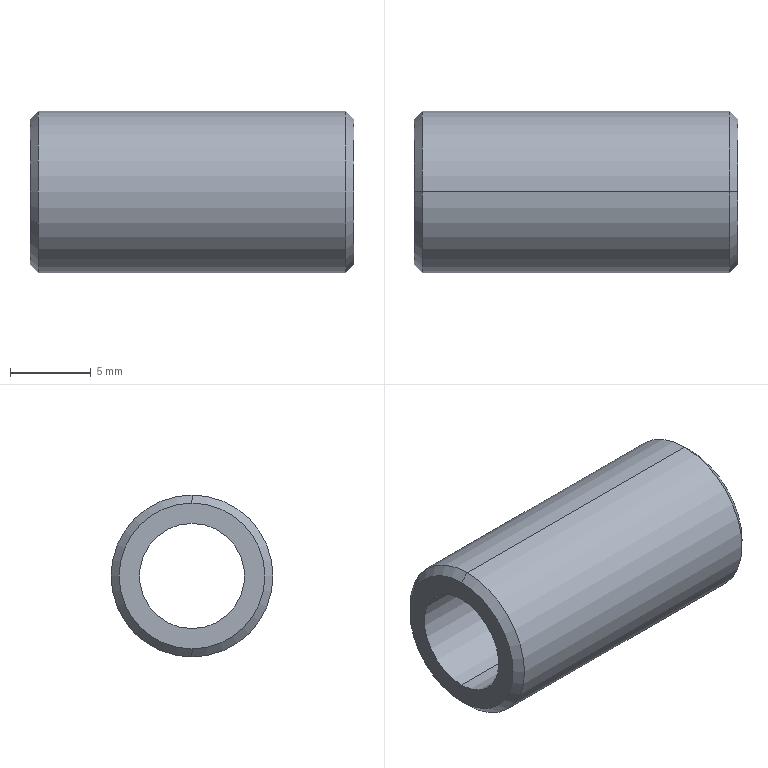Part | SolidWorks | features Chamfer 1, Extrusion 1, ICE 1 | 1 solid | 10 faces | box 20 x 10 x 10 mm | volume 899.543 mm3 | cylinder 4 | cone 4 | plane 2 | commonest cylinder face diameters 6.5 x2 10 x2
STEP:
#1=CARTESIAN_POINT('',(20.,0.,-3.25));
#2=VERTEX_POINT('',#1);
#3=CARTESIAN_POINT('',(20.,0.,3.25));
#4=VERTEX_POINT('',#3);
#5=CARTESIAN_POINT('',(20.,0.,0.));
#6=DIRECTION('',(-1.,0.,0.));
#7=DIRECTION('',(0.,0.,1.));
#8=AXIS2_PLACEMENT_3D('',#5,#6,#7);
#9=CIRCLE('',#8,3.25);
#10=EDGE_CURVE('',#2,#4,#9,.T.);
#11=ORIENTED_EDGE('',*,*,#10,.F.);
#12=CARTESIAN_POINT('',(0.,0.,-3.25));
#13=VERTEX_POINT('',#12);
#14=CARTESIAN_POINT('',(20.,0.,-3.25));
#15=DIRECTION('',(-1.,0.,0.));
#16=VECTOR('',#15,1000.);
#17=LINE('',#14,#16);
#18=EDGE_CURVE('',#2,#13,#17,.T.);
#19=ORIENTED_EDGE('',*,*,#18,.T.);
#20=CARTESIAN_POINT('',(0.,0.,3.25));
#21=VERTEX_POINT('',#20);
#22=CARTESIAN_POINT('',(0.,0.,0.));
#23=DIRECTION('',(-1.,0.,0.));
#24=DIRECTION('',(0.,0.,1.));
#25=AXIS2_PLACEMENT_3D('',#22,#23,#24);
#26=CIRCLE('',#25,3.25);
#27=EDGE_CURVE('',#13,#21,#26,.T.);
#28=ORIENTED_EDGE('',*,*,#27,.T.);
#29=CARTESIAN_POINT('',(20.,0.,3.25));
#30=DIRECTION('',(-1.,0.,0.));
#31=VECTOR('',#30,1000.);
#32=LINE('',#29,#31);
#33=EDGE_CURVE('',#4,#21,#32,.T.);
#34=ORIENTED_EDGE('',*,*,#33,.F.);
#35=EDGE_LOOP('',(#11,#19,#28,#34));
#36=FACE_OUTER_BOUND('',#35,.T.);
#37=CARTESIAN_POINT('',(20.,0.,0.));
#38=DIRECTION('',(-1.,0.,0.));
#39=DIRECTION('',(0.,0.,1.));
#40=AXIS2_PLACEMENT_3D('',#37,#38,#39);
#41=CYLINDRICAL_SURFACE('',#40,3.25);
#42=ADVANCED_FACE('',(#36),#41,.F.);
#43=CARTESIAN_POINT('',(20.,0.,-4.5));
#44=VERTEX_POINT('',#43);
#45=CARTESIAN_POINT('',(20.,0.,4.5));
#46=VERTEX_POINT('',#45);
#47=CARTESIAN_POINT('',(20.,0.,0.));
#48=DIRECTION('',(1.,0.,0.));
#49=DIRECTION('',(0.,0.,-1.));
#50=AXIS2_PLACEMENT_3D('',#47,#48,#49);
#51=CIRCLE('',#50,4.5);
#52=EDGE_CURVE('',#44,#46,#51,.T.);
#53=ORIENTED_EDGE('',*,*,#52,.F.);
#54=CARTESIAN_POINT('',(19.5,0.,-5.));
#55=VERTEX_POINT('',#54);
#56=CARTESIAN_POINT('',(20.,0.,-4.5));
#57=DIRECTION('',(-0.7071,0.,-0.7071));
#58=VECTOR('',#57,1000.);
#59=LINE('',#56,#58);
#60=EDGE_CURVE('',#44,#55,#59,.T.);
#61=ORIENTED_EDGE('',*,*,#60,.T.);
#62=CARTESIAN_POINT('',(19.5,0.,5.));
#63=VERTEX_POINT('',#62);
#64=CARTESIAN_POINT('',(19.5,0.,0.));
#65=DIRECTION('',(-1.,0.,0.));
#66=DIRECTION('',(0.,0.,-1.));
#67=AXIS2_PLACEMENT_3D('',#64,#65,#66);
#68=CIRCLE('',#67,5.);
#69=EDGE_CURVE('',#63,#55,#68,.T.);
#70=ORIENTED_EDGE('',*,*,#69,.F.);
#71=CARTESIAN_POINT('',(20.,0.,4.5));
#72=DIRECTION('',(-0.7071,0.,0.7071));
#73=VECTOR('',#72,1000.);
#74=LINE('',#71,#73);
#75=EDGE_CURVE('',#46,#63,#74,.T.);
#76=ORIENTED_EDGE('',*,*,#75,.F.);
#77=EDGE_LOOP('',(#53,#61,#70,#76));
#78=FACE_OUTER_BOUND('',#77,.T.);
#79=CARTESIAN_POINT('',(20.,0.,0.));
#80=DIRECTION('',(-1.,0.,0.));
#81=DIRECTION('',(0.,0.,1.));
#82=AXIS2_PLACEMENT_3D('',#79,#80,#81);
#83=CONICAL_SURFACE('',#82,4.5,0.7854);
#84=ADVANCED_FACE('',(#78),#83,.T.);
#85=CARTESIAN_POINT('',(0.,0.,4.5));
#86=VERTEX_POINT('',#85);
#87=CARTESIAN_POINT('',(0.,0.,-4.5));
#88=VERTEX_POINT('',#87);
#89=CARTESIAN_POINT('',(0.,0.,0.));
#90=DIRECTION('',(-1.,0.,0.));
#91=DIRECTION('',(0.,0.,-1.));
#92=AXIS2_PLACEMENT_3D('',#89,#90,#91);
#93=CIRCLE('',#92,4.5);
#94=EDGE_CURVE('',#86,#88,#93,.T.);
#95=ORIENTED_EDGE('',*,*,#94,.F.);
#96=CARTESIAN_POINT('',(0.5,0.,5.));
#97=VERTEX_POINT('',#96);
#98=CARTESIAN_POINT('',(0.5,0.,5.));
#99=DIRECTION('',(0.7071,0.,0.7071));
#100=VECTOR('',#99,1000.);
#101=LINE('',#98,#100);
#102=EDGE_CURVE('',#86,#97,#101,.T.);
#103=ORIENTED_EDGE('',*,*,#102,.T.);
#104=CARTESIAN_POINT('',(0.5,0.,-5.));
#105=VERTEX_POINT('',#104);
#106=CARTESIAN_POINT('',(0.5,0.,0.));
#107=DIRECTION('',(1.,0.,0.));
#108=DIRECTION('',(0.,0.,-1.));
#109=AXIS2_PLACEMENT_3D('',#106,#107,#108);
#110=CIRCLE('',#109,5.);
#111=EDGE_CURVE('',#105,#97,#110,.T.);
#112=ORIENTED_EDGE('',*,*,#111,.F.);
#113=CARTESIAN_POINT('',(0.5,0.,-5.));
#114=DIRECTION('',(0.7071,0.,-0.7071));
#115=VECTOR('',#114,1000.);
#116=LINE('',#113,#115);
#117=EDGE_CURVE('',#88,#105,#116,.T.);
#118=ORIENTED_EDGE('',*,*,#117,.F.);
#119=EDGE_LOOP('',(#95,#103,#112,#118));
#120=FACE_OUTER_BOUND('',#119,.T.);
#121=CARTESIAN_POINT('',(0.5,0.,0.));
#122=DIRECTION('',(1.,0.,0.));
#123=DIRECTION('',(0.,0.,-1.));
#124=AXIS2_PLACEMENT_3D('',#121,#122,#123);
#125=CONICAL_SURFACE('',#124,5.,0.7854);
#126=ADVANCED_FACE('',(#120),#125,.T.);
#127=ORIENTED_EDGE('',*,*,#69,.T.);
#128=CARTESIAN_POINT('',(20.,0.,-5.));
#129=DIRECTION('',(-1.,0.,0.));
#130=VECTOR('',#129,1000.);
#131=LINE('',#128,#130);
#132=EDGE_CURVE('',#55,#105,#131,.T.);
#133=ORIENTED_EDGE('',*,*,#132,.T.);
#134=ORIENTED_EDGE('',*,*,#111,.T.);
#135=CARTESIAN_POINT('',(20.,0.,5.));
#136=DIRECTION('',(-1.,0.,0.));
#137=VECTOR('',#136,1000.);
#138=LINE('',#135,#137);
#139=EDGE_CURVE('',#63,#97,#138,.T.);
#140=ORIENTED_EDGE('',*,*,#139,.F.);
#141=EDGE_LOOP('',(#127,#133,#134,#140));
#142=FACE_OUTER_BOUND('',#141,.T.);
#143=CARTESIAN_POINT('',(20.,0.,0.));
#144=DIRECTION('',(-1.,0.,0.));
#145=DIRECTION('',(0.,0.,1.));
#146=AXIS2_PLACEMENT_3D('',#143,#144,#145);
#147=CYLINDRICAL_SURFACE('',#146,5.);
#148=ADVANCED_FACE('',(#142),#147,.T.);
#149=ORIENTED_EDGE('',*,*,#132,.F.);
#150=CARTESIAN_POINT('',(19.5,0.,0.));
#151=DIRECTION('',(-1.,0.,0.));
#152=DIRECTION('',(0.,0.,-1.));
#153=AXIS2_PLACEMENT_3D('',#150,#151,#152);
#154=CIRCLE('',#153,5.);
#155=EDGE_CURVE('',#55,#63,#154,.T.);
#156=ORIENTED_EDGE('',*,*,#155,.T.);
#157=ORIENTED_EDGE('',*,*,#139,.T.);
#158=CARTESIAN_POINT('',(0.5,0.,0.));
#159=DIRECTION('',(1.,0.,0.));
#160=DIRECTION('',(0.,0.,-1.));
#161=AXIS2_PLACEMENT_3D('',#158,#159,#160);
#162=CIRCLE('',#161,5.);
#163=EDGE_CURVE('',#97,#105,#162,.T.);
#164=ORIENTED_EDGE('',*,*,#163,.T.);
#165=EDGE_LOOP('',(#149,#156,#157,#164));
#166=FACE_OUTER_BOUND('',#165,.T.);
#167=CARTESIAN_POINT('',(20.,0.,0.));
#168=DIRECTION('',(-1.,0.,0.));
#169=DIRECTION('',(0.,0.,1.));
#170=AXIS2_PLACEMENT_3D('',#167,#168,#169);
#171=CYLINDRICAL_SURFACE('',#170,5.);
#172=ADVANCED_FACE('',(#166),#171,.T.);
#173=CARTESIAN_POINT('',(20.,0.,0.));
#174=DIRECTION('',(-1.,0.,0.));
#175=DIRECTION('',(0.,0.,1.));
#176=AXIS2_PLACEMENT_3D('',#173,#174,#175);
#177=CIRCLE('',#176,3.25);
#178=EDGE_CURVE('',#4,#2,#177,.T.);
#179=ORIENTED_EDGE('',*,*,#178,.T.);
#180=ORIENTED_EDGE('',*,*,#10,.T.);
#181=EDGE_LOOP('',(#179,#180));
#182=FACE_BOUND('',#181,.T.);
#183=CARTESIAN_POINT('',(20.,0.,0.));
#184=DIRECTION('',(1.,0.,0.));
#185=DIRECTION('',(0.,0.,-1.));
#186=AXIS2_PLACEMENT_3D('',#183,#184,#185);
#187=CIRCLE('',#186,4.5);
#188=EDGE_CURVE('',#46,#44,#187,.T.);
#189=ORIENTED_EDGE('',*,*,#188,.T.);
#190=ORIENTED_EDGE('',*,*,#52,.T.);
#191=EDGE_LOOP('',(#189,#190));
#192=FACE_OUTER_BOUND('',#191,.T.);
#193=CARTESIAN_POINT('',(20.,0.,0.));
#194=DIRECTION('',(1.,0.,0.));
#195=DIRECTION('',(0.,0.,-1.));
#196=AXIS2_PLACEMENT_3D('',#193,#194,#195);
#197=PLANE('',#196);
#198=ADVANCED_FACE('',(#182,#192),#197,.T.);
#199=CARTESIAN_POINT('',(0.,0.,0.));
#200=DIRECTION('',(-1.,0.,0.));
#201=DIRECTION('',(0.,0.,1.));
#202=AXIS2_PLACEMENT_3D('',#199,#200,#201);
#203=CIRCLE('',#202,3.25);
#204=EDGE_CURVE('',#21,#13,#203,.T.);
#205=ORIENTED_EDGE('',*,*,#204,.F.);
#206=ORIENTED_EDGE('',*,*,#27,.F.);
#207=EDGE_LOOP('',(#205,#206));
#208=FACE_BOUND('',#207,.T.);
#209=CARTESIAN_POINT('',(0.,0.,0.));
#210=DIRECTION('',(-1.,0.,0.));
#211=DIRECTION('',(0.,0.,-1.));
#212=AXIS2_PLACEMENT_3D('',#209,#210,#211);
#213=CIRCLE('',#212,4.5);
#214=EDGE_CURVE('',#88,#86,#213,.T.);
#215=ORIENTED_EDGE('',*,*,#214,.T.);
#216=ORIENTED_EDGE('',*,*,#94,.T.);
#217=EDGE_LOOP('',(#215,#216));
#218=FACE_OUTER_BOUND('',#217,.T.);
#219=CARTESIAN_POINT('',(0.,0.,0.));
#220=DIRECTION('',(1.,0.,0.));
#221=DIRECTION('',(0.,0.,-1.));
#222=AXIS2_PLACEMENT_3D('',#219,#220,#221);
#223=PLANE('',#222);
#224=ADVANCED_FACE('',(#208,#218),#223,.F.);
#225=ORIENTED_EDGE('',*,*,#102,.F.);
#226=ORIENTED_EDGE('',*,*,#214,.F.);
#227=ORIENTED_EDGE('',*,*,#117,.T.);
#228=ORIENTED_EDGE('',*,*,#163,.F.);
#229=EDGE_LOOP('',(#225,#226,#227,#228));
#230=FACE_OUTER_BOUND('',#229,.T.);
#231=CARTESIAN_POINT('',(0.5,0.,0.));
#232=DIRECTION('',(1.,0.,0.));
#233=DIRECTION('',(0.,0.,-1.));
#234=AXIS2_PLACEMENT_3D('',#231,#232,#233);
#235=CONICAL_SURFACE('',#234,5.,0.7854);
#236=ADVANCED_FACE('',(#230),#235,.T.);
#237=ORIENTED_EDGE('',*,*,#60,.F.);
#238=ORIENTED_EDGE('',*,*,#188,.F.);
#239=ORIENTED_EDGE('',*,*,#75,.T.);
#240=ORIENTED_EDGE('',*,*,#155,.F.);
#241=EDGE_LOOP('',(#237,#238,#239,#240));
#242=FACE_OUTER_BOUND('',#241,.T.);
#243=CARTESIAN_POINT('',(20.,0.,0.));
#244=DIRECTION('',(-1.,0.,0.));
#245=DIRECTION('',(0.,0.,1.));
#246=AXIS2_PLACEMENT_3D('',#243,#244,#245);
#247=CONICAL_SURFACE('',#246,4.5,0.7854);
#248=ADVANCED_FACE('',(#242),#247,.T.);
#249=ORIENTED_EDGE('',*,*,#18,.F.);
#250=ORIENTED_EDGE('',*,*,#178,.F.);
#251=ORIENTED_EDGE('',*,*,#33,.T.);
#252=ORIENTED_EDGE('',*,*,#204,.T.);
#253=EDGE_LOOP('',(#249,#250,#251,#252));
#254=FACE_OUTER_BOUND('',#253,.T.);
#255=CARTESIAN_POINT('',(20.,0.,0.));
#256=DIRECTION('',(-1.,0.,0.));
#257=DIRECTION('',(0.,0.,1.));
#258=AXIS2_PLACEMENT_3D('',#255,#256,#257);
#259=CYLINDRICAL_SURFACE('',#258,3.25);
#260=ADVANCED_FACE('',(#254),#259,.F.);
#261=CLOSED_SHELL('',(#42,#84,#126,#148,#172,#198,#224,#236,#248,#260));
#262=MANIFOLD_SOLID_BREP('',#261);
#263=CARTESIAN_POINT('',(0.,0.,0.));
#264=DIRECTION('',(0.,0.,1.));
#265=DIRECTION('',(1.,0.,0.));
#266=AXIS2_PLACEMENT_3D('',#263,#264,#265);
#267=(LENGTH_UNIT()NAMED_UNIT(*)SI_UNIT(.MILLI.,.METRE.));
#268=UNCERTAINTY_MEASURE_WITH_UNIT(LENGTH_MEASURE(0.00001),#267,'','');
#269=(NAMED_UNIT(*)PLANE_ANGLE_UNIT()SI_UNIT($,.RADIAN.));
#270=(NAMED_UNIT(*)SI_UNIT($,.STERADIAN.)SOLID_ANGLE_UNIT());
#271=(GEOMETRIC_REPRESENTATION_CONTEXT(3)GLOBAL_UNCERTAINTY_ASSIGNED_CONTEXT((#268))GLOBAL_UNIT_ASSIGNED_CONTEXT((#267,#269,#270))REPRESENTATION_CONTEXT('',''));
#272=ADVANCED_BREP_SHAPE_REPRESENTATION('',(#262,#266),#271);